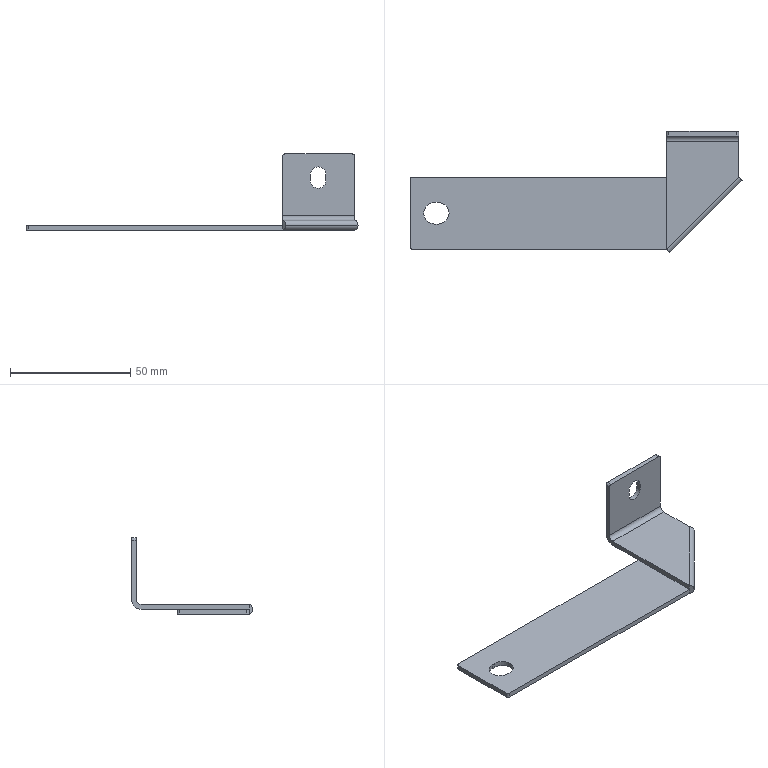Part | NX | features BREP 1 | 1 solid | 32 faces | box 138.159 x 50.414 x 31.629 mm | volume 10937 mm3 | plane 18 | cylinder 14 | commonest cylinder face diameters 2 x4 4 x3 6.5 x3 9 x3 8 x1
STEP:
#1=CARTESIAN_POINT('',(435.713,-98.404,2034.));
#2=VERTEX_POINT('',#1);
#3=CARTESIAN_POINT('',(437.128,-99.818,2036.));
#4=VERTEX_POINT('',#3);
#5=CARTESIAN_POINT('',(435.713,-98.404,2036.));
#6=DIRECTION('',(-0.7071,-0.7071,0.));
#7=DIRECTION('',(0.7071,-0.7071,0.));
#8=AXIS2_PLACEMENT_3D('',#5,#6,#7);
#9=CIRCLE('',#8,2.);
#10=EDGE_CURVE('',#2,#4,#9,.T.);
#11=ORIENTED_EDGE('',*,*,#10,.T.);
#12=CARTESIAN_POINT('',(407.128,-129.818,2036.));
#13=VERTEX_POINT('',#12);
#14=CARTESIAN_POINT('',(437.128,-99.818,2036.));
#15=DIRECTION('',(-0.7071,-0.7071,0.));
#16=VECTOR('',#15,1000.);
#17=LINE('',#14,#16);
#18=EDGE_CURVE('',#4,#13,#17,.T.);
#19=ORIENTED_EDGE('',*,*,#18,.T.);
#20=CARTESIAN_POINT('',(405.713,-128.404,2034.));
#21=VERTEX_POINT('',#20);
#22=CARTESIAN_POINT('',(405.713,-128.404,2036.));
#23=DIRECTION('',(0.7071,0.7071,0.));
#24=DIRECTION('',(0.7071,-0.7071,0.));
#25=AXIS2_PLACEMENT_3D('',#22,#23,#24);
#26=CIRCLE('',#25,2.);
#27=EDGE_CURVE('',#13,#21,#26,.T.);
#28=ORIENTED_EDGE('',*,*,#27,.T.);
#29=CARTESIAN_POINT('',(405.713,-128.404,2034.));
#30=DIRECTION('',(0.7071,0.7071,0.));
#31=VECTOR('',#30,1000.);
#32=LINE('',#29,#31);
#33=EDGE_CURVE('',#21,#2,#32,.T.);
#34=ORIENTED_EDGE('',*,*,#33,.T.);
#35=EDGE_LOOP('',(#11,#19,#28,#34));
#36=FACE_BOUND('',#35,.T.);
#37=CARTESIAN_POINT('',(435.713,-98.404,2036.));
#38=DIRECTION('',(-0.7071,-0.7071,0.));
#39=DIRECTION('',(-0.7071,0.7071,0.));
#40=AXIS2_PLACEMENT_3D('',#37,#38,#39);
#41=CYLINDRICAL_SURFACE('',#40,2.);
#42=ADVANCED_FACE('',(#36),#41,.T.);
#43=CARTESIAN_POINT('',(310.718,-108.904,2034.));
#44=VERTEX_POINT('',#43);
#45=CARTESIAN_POINT('',(315.218,-113.404,2034.));
#46=VERTEX_POINT('',#45);
#47=CARTESIAN_POINT('',(310.718,-113.404,2034.));
#48=DIRECTION('',(0.,0.,-1.));
#49=DIRECTION('',(1.,0.,0.));
#50=AXIS2_PLACEMENT_3D('',#47,#48,#49);
#51=CIRCLE('',#50,4.5);
#52=EDGE_CURVE('',#44,#46,#51,.T.);
#53=ORIENTED_EDGE('',*,*,#52,.T.);
#54=CARTESIAN_POINT('',(315.218,-113.404,2036.));
#55=VERTEX_POINT('',#54);
#56=CARTESIAN_POINT('',(315.218,-113.404,2016.46));
#57=DIRECTION('',(0.,0.,1.));
#58=VECTOR('',#57,1000.);
#59=LINE('',#56,#58);
#60=EDGE_CURVE('',#46,#55,#59,.T.);
#61=ORIENTED_EDGE('',*,*,#60,.T.);
#62=CARTESIAN_POINT('',(310.718,-108.904,2036.));
#63=VERTEX_POINT('',#62);
#64=CARTESIAN_POINT('',(310.718,-113.404,2036.));
#65=DIRECTION('',(0.,0.,-1.));
#66=DIRECTION('',(1.,0.,0.));
#67=AXIS2_PLACEMENT_3D('',#64,#65,#66);
#68=CIRCLE('',#67,4.5);
#69=EDGE_CURVE('',#63,#55,#68,.T.);
#70=ORIENTED_EDGE('',*,*,#69,.F.);
#71=CARTESIAN_POINT('',(310.718,-108.904,2016.46));
#72=DIRECTION('',(0.,0.,1.));
#73=VECTOR('',#72,1000.);
#74=LINE('',#71,#73);
#75=EDGE_CURVE('',#44,#63,#74,.T.);
#76=ORIENTED_EDGE('',*,*,#75,.F.);
#77=EDGE_LOOP('',(#53,#61,#70,#76));
#78=FACE_BOUND('',#77,.T.);
#79=CARTESIAN_POINT('',(310.718,-113.404,2016.46));
#80=DIRECTION('',(0.,0.,1.));
#81=DIRECTION('',(-1.,0.,0.));
#82=AXIS2_PLACEMENT_3D('',#79,#80,#81);
#83=CYLINDRICAL_SURFACE('',#82,4.5);
#84=ADVANCED_FACE('',(#78),#83,.F.);
#85=CARTESIAN_POINT('',(423.779,-81.404,2057.042));
#86=VERTEX_POINT('',#85);
#87=CARTESIAN_POINT('',(420.529,-81.404,2060.292));
#88=VERTEX_POINT('',#87);
#89=CARTESIAN_POINT('',(420.529,-81.404,2057.042));
#90=DIRECTION('',(0.,-1.,0.));
#91=DIRECTION('',(0.,0.,1.));
#92=AXIS2_PLACEMENT_3D('',#89,#90,#91);
#93=CIRCLE('',#92,3.25);
#94=EDGE_CURVE('',#86,#88,#93,.T.);
#95=ORIENTED_EDGE('',*,*,#94,.T.);
#96=CARTESIAN_POINT('',(420.529,-79.404,2060.292));
#97=VERTEX_POINT('',#96);
#98=CARTESIAN_POINT('',(420.529,-80.404,2060.292));
#99=DIRECTION('',(0.,1.,0.));
#100=VECTOR('',#99,1000.);
#101=LINE('',#98,#100);
#102=EDGE_CURVE('',#88,#97,#101,.T.);
#103=ORIENTED_EDGE('',*,*,#102,.T.);
#104=CARTESIAN_POINT('',(423.779,-79.404,2057.042));
#105=VERTEX_POINT('',#104);
#106=CARTESIAN_POINT('',(420.529,-79.404,2057.042));
#107=DIRECTION('',(0.,-1.,0.));
#108=DIRECTION('',(0.,0.,1.));
#109=AXIS2_PLACEMENT_3D('',#106,#107,#108);
#110=CIRCLE('',#109,3.25);
#111=EDGE_CURVE('',#105,#97,#110,.T.);
#112=ORIENTED_EDGE('',*,*,#111,.F.);
#113=CARTESIAN_POINT('',(423.779,-80.404,2057.042));
#114=DIRECTION('',(0.,1.,0.));
#115=VECTOR('',#114,1000.);
#116=LINE('',#113,#115);
#117=EDGE_CURVE('',#86,#105,#116,.T.);
#118=ORIENTED_EDGE('',*,*,#117,.F.);
#119=EDGE_LOOP('',(#95,#103,#112,#118));
#120=FACE_BOUND('',#119,.T.);
#121=CARTESIAN_POINT('',(420.529,-80.404,2057.042));
#122=DIRECTION('',(0.,1.,0.));
#123=DIRECTION('',(0.,0.,-1.));
#124=AXIS2_PLACEMENT_3D('',#121,#122,#123);
#125=CYLINDRICAL_SURFACE('',#124,3.25);
#126=ADVANCED_FACE('',(#120),#125,.F.);
#127=CARTESIAN_POINT('',(298.968,-99.404,2034.));
#128=VERTEX_POINT('',#127);
#129=CARTESIAN_POINT('',(298.968,-127.404,2034.));
#130=VERTEX_POINT('',#129);
#131=CARTESIAN_POINT('',(298.968,-6.11,2034.));
#132=DIRECTION('',(0.,-1.,0.));
#133=VECTOR('',#132,1000.);
#134=LINE('',#131,#133);
#135=EDGE_CURVE('',#128,#130,#134,.T.);
#136=ORIENTED_EDGE('',*,*,#135,.F.);
#137=CARTESIAN_POINT('',(299.968,-98.404,2034.));
#138=VERTEX_POINT('',#137);
#139=CARTESIAN_POINT('',(299.968,-99.404,2034.));
#140=DIRECTION('',(0.,0.,1.));
#141=DIRECTION('',(1.,0.,0.));
#142=AXIS2_PLACEMENT_3D('',#139,#140,#141);
#143=CIRCLE('',#142,1.);
#144=EDGE_CURVE('',#138,#128,#143,.T.);
#145=ORIENTED_EDGE('',*,*,#144,.F.);
#146=CARTESIAN_POINT('',(-23.45,-98.404,2034.));
#147=DIRECTION('',(-1.,0.,0.));
#148=VECTOR('',#147,1000.);
#149=LINE('',#146,#148);
#150=EDGE_CURVE('',#2,#138,#149,.T.);
#151=ORIENTED_EDGE('',*,*,#150,.F.);
#152=ORIENTED_EDGE('',*,*,#33,.F.);
#153=CARTESIAN_POINT('',(299.968,-128.404,2034.));
#154=VERTEX_POINT('',#153);
#155=CARTESIAN_POINT('',(-23.45,-128.404,2034.));
#156=DIRECTION('',(1.,0.,0.));
#157=VECTOR('',#156,1000.);
#158=LINE('',#155,#157);
#159=EDGE_CURVE('',#154,#21,#158,.T.);
#160=ORIENTED_EDGE('',*,*,#159,.F.);
#161=CARTESIAN_POINT('',(299.968,-127.404,2034.));
#162=DIRECTION('',(0.,0.,1.));
#163=DIRECTION('',(1.,0.,0.));
#164=AXIS2_PLACEMENT_3D('',#161,#162,#163);
#165=CIRCLE('',#164,1.);
#166=EDGE_CURVE('',#130,#154,#165,.T.);
#167=ORIENTED_EDGE('',*,*,#166,.F.);
#168=EDGE_LOOP('',(#136,#145,#151,#152,#160,#167));
#169=FACE_BOUND('',#168,.T.);
#170=CARTESIAN_POINT('',(309.218,-117.904,2034.));
#171=VERTEX_POINT('',#170);
#172=CARTESIAN_POINT('',(310.718,-117.904,2034.));
#173=VERTEX_POINT('',#172);
#174=CARTESIAN_POINT('',(309.218,-117.904,2034.));
#175=DIRECTION('',(1.,0.,0.));
#176=VECTOR('',#175,1000.);
#177=LINE('',#174,#176);
#178=EDGE_CURVE('',#171,#173,#177,.T.);
#179=ORIENTED_EDGE('',*,*,#178,.T.);
#180=CARTESIAN_POINT('',(310.718,-113.404,2034.));
#181=DIRECTION('',(0.,0.,-1.));
#182=DIRECTION('',(1.,0.,0.));
#183=AXIS2_PLACEMENT_3D('',#180,#181,#182);
#184=CIRCLE('',#183,4.5);
#185=EDGE_CURVE('',#46,#173,#184,.T.);
#186=ORIENTED_EDGE('',*,*,#185,.F.);
#187=ORIENTED_EDGE('',*,*,#52,.F.);
#188=CARTESIAN_POINT('',(309.218,-108.904,2034.));
#189=VERTEX_POINT('',#188);
#190=CARTESIAN_POINT('',(310.718,-108.904,2034.));
#191=DIRECTION('',(-1.,0.,0.));
#192=VECTOR('',#191,1000.);
#193=LINE('',#190,#192);
#194=EDGE_CURVE('',#44,#189,#193,.T.);
#195=ORIENTED_EDGE('',*,*,#194,.T.);
#196=CARTESIAN_POINT('',(309.218,-113.404,2034.));
#197=DIRECTION('',(0.,0.,-1.));
#198=DIRECTION('',(1.,0.,0.));
#199=AXIS2_PLACEMENT_3D('',#196,#197,#198);
#200=CIRCLE('',#199,4.5);
#201=EDGE_CURVE('',#171,#189,#200,.T.);
#202=ORIENTED_EDGE('',*,*,#201,.F.);
#203=EDGE_LOOP('',(#179,#186,#187,#195,#202));
#204=FACE_BOUND('',#203,.T.);
#205=CARTESIAN_POINT('',(-23.45,-6.11,2034.));
#206=DIRECTION('',(0.,0.,1.));
#207=DIRECTION('',(-1.,0.,0.));
#208=AXIS2_PLACEMENT_3D('',#205,#206,#207);
#209=PLANE('',#208);
#210=ADVANCED_FACE('',(#169,#204),#209,.F.);
#211=ORIENTED_EDGE('',*,*,#135,.T.);
#212=CARTESIAN_POINT('',(298.968,-127.404,2036.));
#213=VERTEX_POINT('',#212);
#214=CARTESIAN_POINT('',(298.968,-127.404,2035.));
#215=DIRECTION('',(0.,0.,1.));
#216=VECTOR('',#215,1000.);
#217=LINE('',#214,#216);
#218=EDGE_CURVE('',#130,#213,#217,.T.);
#219=ORIENTED_EDGE('',*,*,#218,.T.);
#220=CARTESIAN_POINT('',(298.968,-99.404,2036.));
#221=VERTEX_POINT('',#220);
#222=CARTESIAN_POINT('',(298.968,-113.404,2036.));
#223=DIRECTION('',(0.,1.,0.));
#224=VECTOR('',#223,1000.);
#225=LINE('',#222,#224);
#226=EDGE_CURVE('',#213,#221,#225,.T.);
#227=ORIENTED_EDGE('',*,*,#226,.T.);
#228=CARTESIAN_POINT('',(298.968,-99.404,2035.));
#229=DIRECTION('',(0.,0.,-1.));
#230=VECTOR('',#229,1000.);
#231=LINE('',#228,#230);
#232=EDGE_CURVE('',#221,#128,#231,.T.);
#233=ORIENTED_EDGE('',*,*,#232,.T.);
#234=EDGE_LOOP('',(#211,#219,#227,#233));
#235=FACE_BOUND('',#234,.T.);
#236=CARTESIAN_POINT('',(298.968,-113.404,2035.));
#237=DIRECTION('',(-1.,0.,0.));
#238=DIRECTION('',(0.,0.,-1.));
#239=AXIS2_PLACEMENT_3D('',#236,#237,#238);
#240=PLANE('',#239);
#241=ADVANCED_FACE('',(#235),#240,.T.);
#242=CARTESIAN_POINT('',(405.713,-98.404,2036.));
#243=VERTEX_POINT('',#242);
#244=CARTESIAN_POINT('',(435.713,-98.404,2036.));
#245=VERTEX_POINT('',#244);
#246=CARTESIAN_POINT('',(339.341,-98.404,2036.));
#247=DIRECTION('',(1.,0.,0.));
#248=VECTOR('',#247,1000.);
#249=LINE('',#246,#248);
#250=EDGE_CURVE('',#243,#245,#249,.T.);
#251=ORIENTED_EDGE('',*,*,#250,.T.);
#252=CARTESIAN_POINT('',(435.713,-98.404,2035.));
#253=DIRECTION('',(0.,0.,-1.));
#254=VECTOR('',#253,1000.);
#255=LINE('',#252,#254);
#256=EDGE_CURVE('',#245,#2,#255,.T.);
#257=ORIENTED_EDGE('',*,*,#256,.T.);
#258=ORIENTED_EDGE('',*,*,#150,.T.);
#259=CARTESIAN_POINT('',(299.968,-98.404,2036.));
#260=VERTEX_POINT('',#259);
#261=CARTESIAN_POINT('',(299.968,-98.404,2035.));
#262=DIRECTION('',(0.,0.,1.));
#263=VECTOR('',#262,1000.);
#264=LINE('',#261,#263);
#265=EDGE_CURVE('',#138,#260,#264,.T.);
#266=ORIENTED_EDGE('',*,*,#265,.T.);
#267=CARTESIAN_POINT('',(339.341,-98.404,2036.));
#268=DIRECTION('',(1.,0.,0.));
#269=VECTOR('',#268,1000.);
#270=LINE('',#267,#269);
#271=EDGE_CURVE('',#260,#243,#270,.T.);
#272=ORIENTED_EDGE('',*,*,#271,.T.);
#273=EDGE_LOOP('',(#251,#257,#258,#266,#272));
#274=FACE_BOUND('',#273,.T.);
#275=CARTESIAN_POINT('',(339.341,-98.404,2035.));
#276=DIRECTION('',(0.,1.,0.));
#277=DIRECTION('',(0.,0.,-1.));
#278=AXIS2_PLACEMENT_3D('',#275,#276,#277);
#279=PLANE('',#278);
#280=ADVANCED_FACE('',(#274),#279,.T.);
#281=ORIENTED_EDGE('',*,*,#18,.F.);
#282=CARTESIAN_POINT('',(435.713,-98.404,2038.));
#283=VERTEX_POINT('',#282);
#284=CARTESIAN_POINT('',(435.713,-98.404,2036.));
#285=DIRECTION('',(-0.7071,-0.7071,0.));
#286=DIRECTION('',(0.7071,-0.7071,0.));
#287=AXIS2_PLACEMENT_3D('',#284,#285,#286);
#288=CIRCLE('',#287,2.);
#289=EDGE_CURVE('',#4,#283,#288,.T.);
#290=ORIENTED_EDGE('',*,*,#289,.T.);
#291=CARTESIAN_POINT('',(405.713,-128.404,2038.));
#292=VERTEX_POINT('',#291);
#293=CARTESIAN_POINT('',(435.713,-98.404,2038.));
#294=DIRECTION('',(-0.7071,-0.7071,0.));
#295=VECTOR('',#294,1000.);
#296=LINE('',#293,#295);
#297=EDGE_CURVE('',#283,#292,#296,.T.);
#298=ORIENTED_EDGE('',*,*,#297,.T.);
#299=CARTESIAN_POINT('',(405.713,-128.404,2036.));
#300=DIRECTION('',(0.7071,0.7071,0.));
#301=DIRECTION('',(0.7071,-0.7071,0.));
#302=AXIS2_PLACEMENT_3D('',#299,#300,#301);
#303=CIRCLE('',#302,2.);
#304=EDGE_CURVE('',#292,#13,#303,.T.);
#305=ORIENTED_EDGE('',*,*,#304,.T.);
#306=EDGE_LOOP('',(#281,#290,#298,#305));
#307=FACE_BOUND('',#306,.T.);
#308=CARTESIAN_POINT('',(435.713,-98.404,2036.));
#309=DIRECTION('',(-0.7071,-0.7071,0.));
#310=DIRECTION('',(-0.7071,0.7071,0.));
#311=AXIS2_PLACEMENT_3D('',#308,#309,#310);
#312=CYLINDRICAL_SURFACE('',#311,2.);
#313=ADVANCED_FACE('',(#307),#312,.T.);
#314=ORIENTED_EDGE('',*,*,#159,.T.);
#315=CARTESIAN_POINT('',(405.713,-128.404,2036.));
#316=VERTEX_POINT('',#315);
#317=CARTESIAN_POINT('',(405.713,-128.404,2035.));
#318=DIRECTION('',(0.,0.,1.));
#319=VECTOR('',#318,1000.);
#320=LINE('',#317,#319);
#321=EDGE_CURVE('',#21,#316,#320,.T.);
#322=ORIENTED_EDGE('',*,*,#321,.T.);
#323=CARTESIAN_POINT('',(299.968,-128.404,2036.));
#324=VERTEX_POINT('',#323);
#325=CARTESIAN_POINT('',(339.341,-128.404,2036.));
#326=DIRECTION('',(-1.,0.,0.));
#327=VECTOR('',#326,1000.);
#328=LINE('',#325,#327);
#329=EDGE_CURVE('',#316,#324,#328,.T.);
#330=ORIENTED_EDGE('',*,*,#329,.T.);
#331=CARTESIAN_POINT('',(299.968,-128.404,2035.));
#332=DIRECTION('',(0.,0.,-1.));
#333=VECTOR('',#332,1000.);
#334=LINE('',#331,#333);
#335=EDGE_CURVE('',#324,#154,#334,.T.);
#336=ORIENTED_EDGE('',*,*,#335,.T.);
#337=EDGE_LOOP('',(#314,#322,#330,#336));
#338=FACE_BOUND('',#337,.T.);
#339=CARTESIAN_POINT('',(339.341,-128.404,2035.));
#340=DIRECTION('',(0.,-1.,0.));
#341=DIRECTION('',(0.,0.,1.));
#342=AXIS2_PLACEMENT_3D('',#339,#340,#341);
#343=PLANE('',#342);
#344=ADVANCED_FACE('',(#338),#343,.T.);
#345=ORIENTED_EDGE('',*,*,#60,.F.);
#346=ORIENTED_EDGE('',*,*,#185,.T.);
#347=CARTESIAN_POINT('',(310.718,-117.904,2036.));
#348=VERTEX_POINT('',#347);
#349=CARTESIAN_POINT('',(310.718,-117.904,2016.46));
#350=DIRECTION('',(0.,0.,-1.));
#351=VECTOR('',#350,1000.);
#352=LINE('',#349,#351);
#353=EDGE_CURVE('',#348,#173,#352,.T.);
#354=ORIENTED_EDGE('',*,*,#353,.F.);
#355=CARTESIAN_POINT('',(310.718,-113.404,2036.));
#356=DIRECTION('',(0.,0.,-1.));
#357=DIRECTION('',(1.,0.,0.));
#358=AXIS2_PLACEMENT_3D('',#355,#356,#357);
#359=CIRCLE('',#358,4.5);
#360=EDGE_CURVE('',#55,#348,#359,.T.);
#361=ORIENTED_EDGE('',*,*,#360,.F.);
#362=EDGE_LOOP('',(#345,#346,#354,#361));
#363=FACE_BOUND('',#362,.T.);
#364=CARTESIAN_POINT('',(310.718,-113.404,2016.46));
#365=DIRECTION('',(0.,0.,1.));
#366=DIRECTION('',(-1.,0.,0.));
#367=AXIS2_PLACEMENT_3D('',#364,#365,#366);
#368=CYLINDRICAL_SURFACE('',#367,4.5);
#369=ADVANCED_FACE('',(#363),#368,.F.);
#370=ORIENTED_EDGE('',*,*,#201,.T.);
#371=CARTESIAN_POINT('',(309.218,-108.904,2036.));
#372=VERTEX_POINT('',#371);
#373=CARTESIAN_POINT('',(309.218,-108.904,2016.46));
#374=DIRECTION('',(0.,0.,-1.));
#375=VECTOR('',#374,1000.);
#376=LINE('',#373,#375);
#377=EDGE_CURVE('',#372,#189,#376,.T.);
#378=ORIENTED_EDGE('',*,*,#377,.F.);
#379=CARTESIAN_POINT('',(309.218,-117.904,2036.));
#380=VERTEX_POINT('',#379);
#381=CARTESIAN_POINT('',(309.218,-113.404,2036.));
#382=DIRECTION('',(0.,0.,-1.));
#383=DIRECTION('',(1.,0.,0.));
#384=AXIS2_PLACEMENT_3D('',#381,#382,#383);
#385=CIRCLE('',#384,4.5);
#386=EDGE_CURVE('',#380,#372,#385,.T.);
#387=ORIENTED_EDGE('',*,*,#386,.F.);
#388=CARTESIAN_POINT('',(309.218,-117.904,2016.46));
#389=DIRECTION('',(0.,0.,1.));
#390=VECTOR('',#389,1000.);
#391=LINE('',#388,#390);
#392=EDGE_CURVE('',#171,#380,#391,.T.);
#393=ORIENTED_EDGE('',*,*,#392,.F.);
#394=EDGE_LOOP('',(#370,#378,#387,#393));
#395=FACE_BOUND('',#394,.T.);
#396=CARTESIAN_POINT('',(309.218,-113.404,2016.46));
#397=DIRECTION('',(0.,0.,1.));
#398=DIRECTION('',(-1.,0.,0.));
#399=AXIS2_PLACEMENT_3D('',#396,#397,#398);
#400=CYLINDRICAL_SURFACE('',#399,4.5);
#401=ADVANCED_FACE('',(#395),#400,.F.);
#402=ORIENTED_EDGE('',*,*,#218,.F.);
#403=ORIENTED_EDGE('',*,*,#166,.T.);
#404=ORIENTED_EDGE('',*,*,#335,.F.);
#405=CARTESIAN_POINT('',(299.968,-127.404,2036.));
#406=DIRECTION('',(0.,0.,-1.));
#407=DIRECTION('',(1.,0.,0.));
#408=AXIS2_PLACEMENT_3D('',#405,#406,#407);
#409=CIRCLE('',#408,1.);
#410=EDGE_CURVE('',#324,#213,#409,.T.);
#411=ORIENTED_EDGE('',*,*,#410,.T.);
#412=EDGE_LOOP('',(#402,#403,#404,#411));
#413=FACE_BOUND('',#412,.T.);
#414=CARTESIAN_POINT('',(299.968,-127.404,1963.606));
#415=DIRECTION('',(0.,0.,1.));
#416=DIRECTION('',(-1.,0.,0.));
#417=AXIS2_PLACEMENT_3D('',#414,#415,#416);
#418=CYLINDRICAL_SURFACE('',#417,1.);
#419=ADVANCED_FACE('',(#413),#418,.T.);
#420=ORIENTED_EDGE('',*,*,#265,.F.);
#421=ORIENTED_EDGE('',*,*,#144,.T.);
#422=ORIENTED_EDGE('',*,*,#232,.F.);
#423=CARTESIAN_POINT('',(299.968,-99.404,2036.));
#424=DIRECTION('',(0.,0.,-1.));
#425=DIRECTION('',(1.,0.,0.));
#426=AXIS2_PLACEMENT_3D('',#423,#424,#425);
#427=CIRCLE('',#426,1.);
#428=EDGE_CURVE('',#221,#260,#427,.T.);
#429=ORIENTED_EDGE('',*,*,#428,.T.);
#430=EDGE_LOOP('',(#420,#421,#422,#429));
#431=FACE_BOUND('',#430,.T.);
#432=CARTESIAN_POINT('',(299.968,-99.404,1963.606));
#433=DIRECTION('',(0.,0.,1.));
#434=DIRECTION('',(-1.,0.,0.));
#435=AXIS2_PLACEMENT_3D('',#432,#433,#434);
#436=CYLINDRICAL_SURFACE('',#435,1.);
#437=ADVANCED_FACE('',(#431),#436,.T.);
#438=ORIENTED_EDGE('',*,*,#271,.F.);
#439=ORIENTED_EDGE('',*,*,#428,.F.);
#440=ORIENTED_EDGE('',*,*,#226,.F.);
#441=ORIENTED_EDGE('',*,*,#410,.F.);
#442=ORIENTED_EDGE('',*,*,#329,.F.);
#443=CARTESIAN_POINT('',(405.713,-6.11,2036.));
#444=DIRECTION('',(0.,1.,0.));
#445=VECTOR('',#444,1000.);
#446=LINE('',#443,#445);
#447=EDGE_CURVE('',#316,#243,#446,.T.);
#448=ORIENTED_EDGE('',*,*,#447,.T.);
#449=EDGE_LOOP('',(#438,#439,#440,#441,#442,#448));
#450=FACE_BOUND('',#449,.T.);
#451=CARTESIAN_POINT('',(7.55,-117.904,2036.));
#452=DIRECTION('',(-1.,0.,0.));
#453=VECTOR('',#452,1000.);
#454=LINE('',#451,#453);
#455=EDGE_CURVE('',#348,#380,#454,.T.);
#456=ORIENTED_EDGE('',*,*,#455,.T.);
#457=ORIENTED_EDGE('',*,*,#386,.T.);
#458=CARTESIAN_POINT('',(7.55,-108.904,2036.));
#459=DIRECTION('',(1.,0.,0.));
#460=VECTOR('',#459,1000.);
#461=LINE('',#458,#460);
#462=EDGE_CURVE('',#372,#63,#461,.T.);
#463=ORIENTED_EDGE('',*,*,#462,.T.);
#464=ORIENTED_EDGE('',*,*,#69,.T.);
#465=ORIENTED_EDGE('',*,*,#360,.T.);
#466=EDGE_LOOP('',(#456,#457,#463,#464,#465));
#467=FACE_BOUND('',#466,.T.);
#468=CARTESIAN_POINT('',(7.55,-6.11,2036.));
#469=DIRECTION('',(0.,0.,1.));
#470=DIRECTION('',(-1.,0.,0.));
#471=AXIS2_PLACEMENT_3D('',#468,#469,#470);
#472=PLANE('',#471);
#473=ADVANCED_FACE('',(#450,#467),#472,.T.);
#474=CARTESIAN_POINT('',(435.713,-98.404,2036.));
#475=DIRECTION('',(0.,0.,1.));
#476=VECTOR('',#475,1000.);
#477=LINE('',#474,#476);
#478=EDGE_CURVE('',#245,#283,#477,.T.);
#479=ORIENTED_EDGE('',*,*,#478,.T.);
#480=ORIENTED_EDGE('',*,*,#289,.F.);
#481=ORIENTED_EDGE('',*,*,#10,.F.);
#482=ORIENTED_EDGE('',*,*,#256,.F.);
#483=EDGE_LOOP('',(#479,#480,#481,#482));
#484=FACE_BOUND('',#483,.T.);
#485=CARTESIAN_POINT('',(436.42,-99.111,2036.));
#486=DIRECTION('',(0.7071,0.7071,0.));
#487=DIRECTION('',(0.7071,-0.7071,0.));
#488=AXIS2_PLACEMENT_3D('',#485,#486,#487);
#489=PLANE('',#488);
#490=ADVANCED_FACE('',(#484),#489,.T.);
#491=CARTESIAN_POINT('',(435.713,-83.404,2036.));
#492=VERTEX_POINT('',#491);
#493=CARTESIAN_POINT('',(435.713,-6.11,2036.));
#494=DIRECTION('',(0.,1.,0.));
#495=VECTOR('',#494,1000.);
#496=LINE('',#493,#495);
#497=EDGE_CURVE('',#245,#492,#496,.T.);
#498=ORIENTED_EDGE('',*,*,#497,.F.);
#499=ORIENTED_EDGE('',*,*,#250,.F.);
#500=CARTESIAN_POINT('',(405.713,-83.404,2036.));
#501=VERTEX_POINT('',#500);
#502=CARTESIAN_POINT('',(405.713,-6.11,2036.));
#503=DIRECTION('',(0.,-1.,0.));
#504=VECTOR('',#503,1000.);
#505=LINE('',#502,#504);
#506=EDGE_CURVE('',#501,#243,#505,.T.);
#507=ORIENTED_EDGE('',*,*,#506,.F.);
#508=CARTESIAN_POINT('',(7.55,-83.404,2036.));
#509=DIRECTION('',(-1.,0.,0.));
#510=VECTOR('',#509,1000.);
#511=LINE('',#508,#510);
#512=EDGE_CURVE('',#492,#501,#511,.T.);
#513=ORIENTED_EDGE('',*,*,#512,.F.);
#514=EDGE_LOOP('',(#498,#499,#507,#513));
#515=FACE_BOUND('',#514,.T.);
#516=CARTESIAN_POINT('',(7.55,-6.11,2036.));
#517=DIRECTION('',(0.,0.,1.));
#518=DIRECTION('',(-1.,0.,0.));
#519=AXIS2_PLACEMENT_3D('',#516,#517,#518);
#520=PLANE('',#519);
#521=ADVANCED_FACE('',(#515),#520,.F.);
#522=ORIENTED_EDGE('',*,*,#304,.F.);
#523=CARTESIAN_POINT('',(405.713,-128.404,2036.));
#524=DIRECTION('',(0.,0.,-1.));
#525=VECTOR('',#524,1000.);
#526=LINE('',#523,#525);
#527=EDGE_CURVE('',#292,#316,#526,.T.);
#528=ORIENTED_EDGE('',*,*,#527,.T.);
#529=ORIENTED_EDGE('',*,*,#321,.F.);
#530=ORIENTED_EDGE('',*,*,#27,.F.);
#531=EDGE_LOOP('',(#522,#528,#529,#530));
#532=FACE_BOUND('',#531,.T.);
#533=CARTESIAN_POINT('',(406.42,-129.111,2036.));
#534=DIRECTION('',(-0.7071,-0.7071,0.));
#535=DIRECTION('',(-0.7071,0.7071,0.));
#536=AXIS2_PLACEMENT_3D('',#533,#534,#535);
#537=PLANE('',#536);
#538=ADVANCED_FACE('',(#532),#537,.T.);
#539=ORIENTED_EDGE('',*,*,#353,.T.);
#540=ORIENTED_EDGE('',*,*,#178,.F.);
#541=ORIENTED_EDGE('',*,*,#392,.T.);
#542=ORIENTED_EDGE('',*,*,#455,.F.);
#543=EDGE_LOOP('',(#539,#540,#541,#542));
#544=FACE_BOUND('',#543,.T.);
#545=CARTESIAN_POINT('',(309.218,-117.904,2016.46));
#546=DIRECTION('',(0.,-1.,0.));
#547=DIRECTION('',(0.,0.,1.));
#548=AXIS2_PLACEMENT_3D('',#545,#546,#547);
#549=PLANE('',#548);
#550=ADVANCED_FACE('',(#544),#549,.F.);
#551=ORIENTED_EDGE('',*,*,#377,.T.);
#552=ORIENTED_EDGE('',*,*,#194,.F.);
#553=ORIENTED_EDGE('',*,*,#75,.T.);
#554=ORIENTED_EDGE('',*,*,#462,.F.);
#555=EDGE_LOOP('',(#551,#552,#553,#554));
#556=FACE_BOUND('',#555,.T.);
#557=CARTESIAN_POINT('',(310.718,-108.904,2016.46));
#558=DIRECTION('',(0.,1.,0.));
#559=DIRECTION('',(0.,0.,-1.));
#560=AXIS2_PLACEMENT_3D('',#557,#558,#559);
#561=PLANE('',#560);
#562=ADVANCED_FACE('',(#556),#561,.F.);
#563=CARTESIAN_POINT('',(405.713,-83.404,2038.));
#564=VERTEX_POINT('',#563);
#565=CARTESIAN_POINT('',(405.713,-103.904,2038.));
#566=DIRECTION('',(0.,1.,0.));
#567=VECTOR('',#566,1000.);
#568=LINE('',#565,#567);
#569=EDGE_CURVE('',#292,#564,#568,.T.);
#570=ORIENTED_EDGE('',*,*,#569,.T.);
#571=CARTESIAN_POINT('',(405.713,-81.404,2040.));
#572=VERTEX_POINT('',#571);
#573=CARTESIAN_POINT('',(405.713,-83.404,2040.));
#574=DIRECTION('',(1.,0.,0.));
#575=DIRECTION('',(0.,0.,1.));
#576=AXIS2_PLACEMENT_3D('',#573,#574,#575);
#577=CIRCLE('',#576,2.);
#578=EDGE_CURVE('',#564,#572,#577,.T.);
#579=ORIENTED_EDGE('',*,*,#578,.T.);
#580=CARTESIAN_POINT('',(405.713,-81.404,2064.629));
#581=VERTEX_POINT('',#580);
#582=CARTESIAN_POINT('',(405.713,-81.404,2034.5));
#583=DIRECTION('',(0.,0.,1.));
#584=VECTOR('',#583,1000.);
#585=LINE('',#582,#584);
#586=EDGE_CURVE('',#572,#581,#585,.T.);
#587=ORIENTED_EDGE('',*,*,#586,.T.);
#588=CARTESIAN_POINT('',(405.713,-79.404,2064.629));
#589=VERTEX_POINT('',#588);
#590=CARTESIAN_POINT('',(405.713,-103.904,2064.629));
#591=DIRECTION('',(0.,1.,0.));
#592=VECTOR('',#591,1000.);
#593=LINE('',#590,#592);
#594=EDGE_CURVE('',#581,#589,#593,.T.);
#595=ORIENTED_EDGE('',*,*,#594,.T.);
#596=CARTESIAN_POINT('',(405.713,-79.404,2040.));
#597=VERTEX_POINT('',#596);
#598=CARTESIAN_POINT('',(405.713,-79.404,2034.5));
#599=DIRECTION('',(0.,0.,-1.));
#600=VECTOR('',#599,1000.);
#601=LINE('',#598,#600);
#602=EDGE_CURVE('',#589,#597,#601,.T.);
#603=ORIENTED_EDGE('',*,*,#602,.T.);
#604=CARTESIAN_POINT('',(405.713,-83.404,2040.));
#605=DIRECTION('',(-1.,0.,0.));
#606=DIRECTION('',(0.,0.,1.));
#607=AXIS2_PLACEMENT_3D('',#604,#605,#606);
#608=CIRCLE('',#607,4.);
#609=EDGE_CURVE('',#597,#501,#608,.T.);
#610=ORIENTED_EDGE('',*,*,#609,.T.);
#611=ORIENTED_EDGE('',*,*,#506,.T.);
#612=ORIENTED_EDGE('',*,*,#447,.F.);
#613=ORIENTED_EDGE('',*,*,#527,.F.);
#614=EDGE_LOOP('',(#570,#579,#587,#595,#603,#610,#611,#612,#613));
#615=FACE_BOUND('',#614,.T.);
#616=CARTESIAN_POINT('',(405.713,-103.904,2034.5));
#617=DIRECTION('',(-1.,0.,0.));
#618=DIRECTION('',(0.,0.,-1.));
#619=AXIS2_PLACEMENT_3D('',#616,#617,#618);
#620=PLANE('',#619);
#621=ADVANCED_FACE('',(#615),#620,.T.);
#622=CARTESIAN_POINT('',(435.713,-83.404,2038.));
#623=VERTEX_POINT('',#622);
#624=CARTESIAN_POINT('',(435.713,-88.904,2038.));
#625=DIRECTION('',(0.,-1.,0.));
#626=VECTOR('',#625,1000.);
#627=LINE('',#624,#626);
#628=EDGE_CURVE('',#623,#283,#627,.T.);
#629=ORIENTED_EDGE('',*,*,#628,.T.);
#630=ORIENTED_EDGE('',*,*,#478,.F.);
#631=ORIENTED_EDGE('',*,*,#497,.T.);
#632=CARTESIAN_POINT('',(435.713,-79.404,2040.));
#633=VERTEX_POINT('',#632);
#634=CARTESIAN_POINT('',(435.713,-83.404,2040.));
#635=DIRECTION('',(1.,0.,0.));
#636=DIRECTION('',(0.,0.,1.));
#637=AXIS2_PLACEMENT_3D('',#634,#635,#636);
#638=CIRCLE('',#637,4.);
#639=EDGE_CURVE('',#492,#633,#638,.T.);
#640=ORIENTED_EDGE('',*,*,#639,.T.);
#641=CARTESIAN_POINT('',(435.713,-79.404,2064.629));
#642=VERTEX_POINT('',#641);
#643=CARTESIAN_POINT('',(435.713,-79.404,2034.5));
#644=DIRECTION('',(0.,0.,1.));
#645=VECTOR('',#644,1000.);
#646=LINE('',#643,#645);
#647=EDGE_CURVE('',#633,#642,#646,.T.);
#648=ORIENTED_EDGE('',*,*,#647,.T.);
#649=CARTESIAN_POINT('',(435.713,-81.404,2064.629));
#650=VERTEX_POINT('',#649);
#651=CARTESIAN_POINT('',(435.713,-88.904,2064.629));
#652=DIRECTION('',(0.,-1.,0.));
#653=VECTOR('',#652,1000.);
#654=LINE('',#651,#653);
#655=EDGE_CURVE('',#642,#650,#654,.T.);
#656=ORIENTED_EDGE('',*,*,#655,.T.);
#657=CARTESIAN_POINT('',(435.713,-81.404,2040.));
#658=VERTEX_POINT('',#657);
#659=CARTESIAN_POINT('',(435.713,-81.404,2034.5));
#660=DIRECTION('',(0.,0.,-1.));
#661=VECTOR('',#660,1000.);
#662=LINE('',#659,#661);
#663=EDGE_CURVE('',#650,#658,#662,.T.);
#664=ORIENTED_EDGE('',*,*,#663,.T.);
#665=CARTESIAN_POINT('',(435.713,-83.404,2040.));
#666=DIRECTION('',(-1.,0.,0.));
#667=DIRECTION('',(0.,0.,1.));
#668=AXIS2_PLACEMENT_3D('',#665,#666,#667);
#669=CIRCLE('',#668,2.);
#670=EDGE_CURVE('',#658,#623,#669,.T.);
#671=ORIENTED_EDGE('',*,*,#670,.T.);
#672=EDGE_LOOP('',(#629,#630,#631,#640,#648,#656,#664,#671));
#673=FACE_BOUND('',#672,.T.);
#674=CARTESIAN_POINT('',(435.713,-88.904,2034.5));
#675=DIRECTION('',(1.,0.,0.));
#676=DIRECTION('',(0.,0.,1.));
#677=AXIS2_PLACEMENT_3D('',#674,#675,#676);
#678=PLANE('',#677);
#679=ADVANCED_FACE('',(#673),#678,.T.);
#680=ORIENTED_EDGE('',*,*,#512,.T.);
#681=ORIENTED_EDGE('',*,*,#609,.F.);
#682=CARTESIAN_POINT('',(435.713,-79.404,2040.));
#683=DIRECTION('',(1.,0.,0.));
#684=VECTOR('',#683,1000.);
#685=LINE('',#682,#684);
#686=EDGE_CURVE('',#597,#633,#685,.T.);
#687=ORIENTED_EDGE('',*,*,#686,.T.);
#688=ORIENTED_EDGE('',*,*,#639,.F.);
#689=EDGE_LOOP('',(#680,#681,#687,#688));
#690=FACE_BOUND('',#689,.T.);
#691=CARTESIAN_POINT('',(435.713,-83.404,2040.));
#692=DIRECTION('',(-1.,0.,0.));
#693=DIRECTION('',(0.,0.,-1.));
#694=AXIS2_PLACEMENT_3D('',#691,#692,#693);
#695=CYLINDRICAL_SURFACE('',#694,4.);
#696=ADVANCED_FACE('',(#690),#695,.T.);
#697=ORIENTED_EDGE('',*,*,#297,.F.);
#698=ORIENTED_EDGE('',*,*,#628,.F.);
#699=CARTESIAN_POINT('',(412.841,-83.404,2038.));
#700=DIRECTION('',(1.,0.,0.));
#701=VECTOR('',#700,1000.);
#702=LINE('',#699,#701);
#703=EDGE_CURVE('',#564,#623,#702,.T.);
#704=ORIENTED_EDGE('',*,*,#703,.F.);
#705=ORIENTED_EDGE('',*,*,#569,.F.);
#706=EDGE_LOOP('',(#697,#698,#704,#705));
#707=FACE_BOUND('',#706,.T.);
#708=CARTESIAN_POINT('',(412.841,-121.276,2038.));
#709=DIRECTION('',(0.,0.,-1.));
#710=DIRECTION('',(1.,0.,0.));
#711=AXIS2_PLACEMENT_3D('',#708,#709,#710);
#712=PLANE('',#711);
#713=ADVANCED_FACE('',(#707),#712,.F.);
#714=ORIENTED_EDGE('',*,*,#578,.F.);
#715=ORIENTED_EDGE('',*,*,#703,.T.);
#716=ORIENTED_EDGE('',*,*,#670,.F.);
#717=CARTESIAN_POINT('',(435.713,-81.404,2040.));
#718=DIRECTION('',(1.,0.,0.));
#719=VECTOR('',#718,1000.);
#720=LINE('',#717,#719);
#721=EDGE_CURVE('',#572,#658,#720,.T.);
#722=ORIENTED_EDGE('',*,*,#721,.F.);
#723=EDGE_LOOP('',(#714,#715,#716,#722));
#724=FACE_BOUND('',#723,.T.);
#725=CARTESIAN_POINT('',(435.713,-83.404,2040.));
#726=DIRECTION('',(-1.,0.,0.));
#727=DIRECTION('',(0.,0.,-1.));
#728=AXIS2_PLACEMENT_3D('',#725,#726,#727);
#729=CYLINDRICAL_SURFACE('',#728,2.);
#730=ADVANCED_FACE('',(#724),#729,.F.);
#731=ORIENTED_EDGE('',*,*,#602,.F.);
#732=CARTESIAN_POINT('',(406.713,-79.404,2065.629));
#733=VERTEX_POINT('',#732);
#734=CARTESIAN_POINT('',(406.713,-79.404,2064.629));
#735=DIRECTION('',(0.,1.,0.));
#736=DIRECTION('',(0.,0.,-1.));
#737=AXIS2_PLACEMENT_3D('',#734,#735,#736);
#738=CIRCLE('',#737,1.);
#739=EDGE_CURVE('',#589,#733,#738,.T.);
#740=ORIENTED_EDGE('',*,*,#739,.T.);
#741=CARTESIAN_POINT('',(434.713,-79.404,2065.629));
#742=VERTEX_POINT('',#741);
#743=CARTESIAN_POINT('',(405.713,-79.404,2065.629));
#744=DIRECTION('',(1.,0.,0.));
#745=VECTOR('',#744,1000.);
#746=LINE('',#743,#745);
#747=EDGE_CURVE('',#733,#742,#746,.T.);
#748=ORIENTED_EDGE('',*,*,#747,.T.);
#749=CARTESIAN_POINT('',(434.713,-79.404,2064.629));
#750=DIRECTION('',(0.,1.,0.));
#751=DIRECTION('',(0.,0.,1.));
#752=AXIS2_PLACEMENT_3D('',#749,#750,#751);
#753=CIRCLE('',#752,1.);
#754=EDGE_CURVE('',#742,#642,#753,.T.);
#755=ORIENTED_EDGE('',*,*,#754,.T.);
#756=ORIENTED_EDGE('',*,*,#647,.F.);
#757=ORIENTED_EDGE('',*,*,#686,.F.);
#758=EDGE_LOOP('',(#731,#740,#748,#755,#756,#757));
#759=FACE_BOUND('',#758,.T.);
#760=CARTESIAN_POINT('',(417.279,-79.404,2057.042));
#761=VERTEX_POINT('',#760);
#762=CARTESIAN_POINT('',(417.279,-79.404,2054.542));
#763=VERTEX_POINT('',#762);
#764=CARTESIAN_POINT('',(417.279,-79.404,2033.5));
#765=DIRECTION('',(0.,0.,-1.));
#766=VECTOR('',#765,1000.);
#767=LINE('',#764,#766);
#768=EDGE_CURVE('',#761,#763,#767,.T.);
#769=ORIENTED_EDGE('',*,*,#768,.T.);
#770=CARTESIAN_POINT('',(423.779,-79.404,2054.542));
#771=VERTEX_POINT('',#770);
#772=CARTESIAN_POINT('',(420.529,-79.404,2054.542));
#773=DIRECTION('',(0.,-1.,0.));
#774=DIRECTION('',(0.,0.,1.));
#775=AXIS2_PLACEMENT_3D('',#772,#773,#774);
#776=CIRCLE('',#775,3.25);
#777=EDGE_CURVE('',#763,#771,#776,.T.);
#778=ORIENTED_EDGE('',*,*,#777,.T.);
#779=CARTESIAN_POINT('',(423.779,-79.404,2033.5));
#780=DIRECTION('',(0.,0.,1.));
#781=VECTOR('',#780,1000.);
#782=LINE('',#779,#781);
#783=EDGE_CURVE('',#771,#105,#782,.T.);
#784=ORIENTED_EDGE('',*,*,#783,.T.);
#785=ORIENTED_EDGE('',*,*,#111,.T.);
#786=CARTESIAN_POINT('',(420.529,-79.404,2057.042));
#787=DIRECTION('',(0.,-1.,0.));
#788=DIRECTION('',(0.,0.,1.));
#789=AXIS2_PLACEMENT_3D('',#786,#787,#788);
#790=CIRCLE('',#789,3.25);
#791=EDGE_CURVE('',#97,#761,#790,.T.);
#792=ORIENTED_EDGE('',*,*,#791,.T.);
#793=EDGE_LOOP('',(#769,#778,#784,#785,#792));
#794=FACE_BOUND('',#793,.T.);
#795=CARTESIAN_POINT('',(405.713,-79.404,2033.5));
#796=DIRECTION('',(0.,1.,0.));
#797=DIRECTION('',(0.,0.,-1.));
#798=AXIS2_PLACEMENT_3D('',#795,#796,#797);
#799=PLANE('',#798);
#800=ADVANCED_FACE('',(#759,#794),#799,.T.);
#801=CARTESIAN_POINT('',(406.713,-81.404,2065.629));
#802=VERTEX_POINT('',#801);
#803=CARTESIAN_POINT('',(406.713,-81.404,2064.629));
#804=DIRECTION('',(0.,1.,0.));
#805=DIRECTION('',(0.,0.,-1.));
#806=AXIS2_PLACEMENT_3D('',#803,#804,#805);
#807=CIRCLE('',#806,1.);
#808=EDGE_CURVE('',#581,#802,#807,.T.);
#809=ORIENTED_EDGE('',*,*,#808,.T.);
#810=CARTESIAN_POINT('',(406.713,-103.904,2065.629));
#811=DIRECTION('',(0.,1.,0.));
#812=VECTOR('',#811,1000.);
#813=LINE('',#810,#812);
#814=EDGE_CURVE('',#802,#733,#813,.T.);
#815=ORIENTED_EDGE('',*,*,#814,.T.);
#816=ORIENTED_EDGE('',*,*,#739,.F.);
#817=ORIENTED_EDGE('',*,*,#594,.F.);
#818=EDGE_LOOP('',(#809,#815,#816,#817));
#819=FACE_BOUND('',#818,.T.);
#820=CARTESIAN_POINT('',(406.713,-103.904,2064.629));
#821=DIRECTION('',(0.,-1.,0.));
#822=DIRECTION('',(0.,0.,1.));
#823=AXIS2_PLACEMENT_3D('',#820,#821,#822);
#824=CYLINDRICAL_SURFACE('',#823,1.);
#825=ADVANCED_FACE('',(#819),#824,.T.);
#826=ORIENTED_EDGE('',*,*,#808,.F.);
#827=ORIENTED_EDGE('',*,*,#586,.F.);
#828=ORIENTED_EDGE('',*,*,#721,.T.);
#829=ORIENTED_EDGE('',*,*,#663,.F.);
#830=CARTESIAN_POINT('',(434.713,-81.404,2065.629));
#831=VERTEX_POINT('',#830);
#832=CARTESIAN_POINT('',(434.713,-81.404,2064.629));
#833=DIRECTION('',(0.,1.,0.));
#834=DIRECTION('',(0.,0.,1.));
#835=AXIS2_PLACEMENT_3D('',#832,#833,#834);
#836=CIRCLE('',#835,1.);
#837=EDGE_CURVE('',#831,#650,#836,.T.);
#838=ORIENTED_EDGE('',*,*,#837,.F.);
#839=CARTESIAN_POINT('',(405.713,-81.404,2065.629));
#840=DIRECTION('',(1.,0.,0.));
#841=VECTOR('',#840,1000.);
#842=LINE('',#839,#841);
#843=EDGE_CURVE('',#802,#831,#842,.T.);
#844=ORIENTED_EDGE('',*,*,#843,.F.);
#845=EDGE_LOOP('',(#826,#827,#828,#829,#838,#844));
#846=FACE_BOUND('',#845,.T.);
#847=CARTESIAN_POINT('',(417.279,-81.404,2057.042));
#848=VERTEX_POINT('',#847);
#849=CARTESIAN_POINT('',(417.279,-81.404,2054.542));
#850=VERTEX_POINT('',#849);
#851=CARTESIAN_POINT('',(417.279,-81.404,2033.5));
#852=DIRECTION('',(0.,0.,-1.));
#853=VECTOR('',#852,1000.);
#854=LINE('',#851,#853);
#855=EDGE_CURVE('',#848,#850,#854,.T.);
#856=ORIENTED_EDGE('',*,*,#855,.F.);
#857=CARTESIAN_POINT('',(420.529,-81.404,2057.042));
#858=DIRECTION('',(0.,-1.,0.));
#859=DIRECTION('',(0.,0.,1.));
#860=AXIS2_PLACEMENT_3D('',#857,#858,#859);
#861=CIRCLE('',#860,3.25);
#862=EDGE_CURVE('',#88,#848,#861,.T.);
#863=ORIENTED_EDGE('',*,*,#862,.F.);
#864=ORIENTED_EDGE('',*,*,#94,.F.);
#865=CARTESIAN_POINT('',(423.779,-81.404,2054.542));
#866=VERTEX_POINT('',#865);
#867=CARTESIAN_POINT('',(423.779,-81.404,2033.5));
#868=DIRECTION('',(0.,0.,1.));
#869=VECTOR('',#868,1000.);
#870=LINE('',#867,#869);
#871=EDGE_CURVE('',#866,#86,#870,.T.);
#872=ORIENTED_EDGE('',*,*,#871,.F.);
#873=CARTESIAN_POINT('',(420.529,-81.404,2054.542));
#874=DIRECTION('',(0.,-1.,0.));
#875=DIRECTION('',(0.,0.,1.));
#876=AXIS2_PLACEMENT_3D('',#873,#874,#875);
#877=CIRCLE('',#876,3.25);
#878=EDGE_CURVE('',#850,#866,#877,.T.);
#879=ORIENTED_EDGE('',*,*,#878,.F.);
#880=EDGE_LOOP('',(#856,#863,#864,#872,#879));
#881=FACE_BOUND('',#880,.T.);
#882=CARTESIAN_POINT('',(405.713,-81.404,2033.5));
#883=DIRECTION('',(0.,1.,0.));
#884=DIRECTION('',(0.,0.,-1.));
#885=AXIS2_PLACEMENT_3D('',#882,#883,#884);
#886=PLANE('',#885);
#887=ADVANCED_FACE('',(#846,#881),#886,.F.);
#888=ORIENTED_EDGE('',*,*,#754,.F.);
#889=CARTESIAN_POINT('',(434.713,-80.404,2065.629));
#890=DIRECTION('',(0.,-1.,0.));
#891=VECTOR('',#890,1000.);
#892=LINE('',#889,#891);
#893=EDGE_CURVE('',#742,#831,#892,.T.);
#894=ORIENTED_EDGE('',*,*,#893,.T.);
#895=ORIENTED_EDGE('',*,*,#837,.T.);
#896=ORIENTED_EDGE('',*,*,#655,.F.);
#897=EDGE_LOOP('',(#888,#894,#895,#896));
#898=FACE_BOUND('',#897,.T.);
#899=CARTESIAN_POINT('',(434.713,-80.404,2064.629));
#900=DIRECTION('',(0.,1.,0.));
#901=DIRECTION('',(0.,0.,-1.));
#902=AXIS2_PLACEMENT_3D('',#899,#900,#901);
#903=CYLINDRICAL_SURFACE('',#902,1.);
#904=ADVANCED_FACE('',(#898),#903,.T.);
#905=ORIENTED_EDGE('',*,*,#747,.F.);
#906=ORIENTED_EDGE('',*,*,#814,.F.);
#907=ORIENTED_EDGE('',*,*,#843,.T.);
#908=ORIENTED_EDGE('',*,*,#893,.F.);
#909=EDGE_LOOP('',(#905,#906,#907,#908));
#910=FACE_BOUND('',#909,.T.);
#911=CARTESIAN_POINT('',(420.713,-80.404,2065.629));
#912=DIRECTION('',(0.,0.,1.));
#913=DIRECTION('',(-1.,0.,0.));
#914=AXIS2_PLACEMENT_3D('',#911,#912,#913);
#915=PLANE('',#914);
#916=ADVANCED_FACE('',(#910),#915,.T.);
#917=CARTESIAN_POINT('',(417.279,-80.404,2054.542));
#918=DIRECTION('',(0.,1.,0.));
#919=VECTOR('',#918,1000.);
#920=LINE('',#917,#919);
#921=EDGE_CURVE('',#850,#763,#920,.T.);
#922=ORIENTED_EDGE('',*,*,#921,.F.);
#923=ORIENTED_EDGE('',*,*,#878,.T.);
#924=CARTESIAN_POINT('',(423.779,-80.404,2054.542));
#925=DIRECTION('',(0.,-1.,0.));
#926=VECTOR('',#925,1000.);
#927=LINE('',#924,#926);
#928=EDGE_CURVE('',#771,#866,#927,.T.);
#929=ORIENTED_EDGE('',*,*,#928,.F.);
#930=ORIENTED_EDGE('',*,*,#777,.F.);
#931=EDGE_LOOP('',(#922,#923,#929,#930));
#932=FACE_BOUND('',#931,.T.);
#933=CARTESIAN_POINT('',(420.529,-80.404,2054.542));
#934=DIRECTION('',(0.,1.,0.));
#935=DIRECTION('',(0.,0.,-1.));
#936=AXIS2_PLACEMENT_3D('',#933,#934,#935);
#937=CYLINDRICAL_SURFACE('',#936,3.25);
#938=ADVANCED_FACE('',(#932),#937,.F.);
#939=ORIENTED_EDGE('',*,*,#768,.F.);
#940=CARTESIAN_POINT('',(417.279,-81.404,2057.042));
#941=DIRECTION('',(0.,-1.,0.));
#942=VECTOR('',#941,1000.);
#943=LINE('',#940,#942);
#944=EDGE_CURVE('',#761,#848,#943,.T.);
#945=ORIENTED_EDGE('',*,*,#944,.T.);
#946=ORIENTED_EDGE('',*,*,#855,.T.);
#947=ORIENTED_EDGE('',*,*,#921,.T.);
#948=EDGE_LOOP('',(#939,#945,#946,#947));
#949=FACE_BOUND('',#948,.T.);
#950=CARTESIAN_POINT('',(417.279,-81.404,2060.292));
#951=DIRECTION('',(1.,0.,0.));
#952=DIRECTION('',(0.,0.,1.));
#953=AXIS2_PLACEMENT_3D('',#950,#951,#952);
#954=PLANE('',#953);
#955=ADVANCED_FACE('',(#949),#954,.T.);
#956=ORIENTED_EDGE('',*,*,#102,.F.);
#957=ORIENTED_EDGE('',*,*,#862,.T.);
#958=ORIENTED_EDGE('',*,*,#944,.F.);
#959=ORIENTED_EDGE('',*,*,#791,.F.);
#960=EDGE_LOOP('',(#956,#957,#958,#959));
#961=FACE_BOUND('',#960,.T.);
#962=CARTESIAN_POINT('',(420.529,-80.404,2057.042));
#963=DIRECTION('',(0.,1.,0.));
#964=DIRECTION('',(0.,0.,-1.));
#965=AXIS2_PLACEMENT_3D('',#962,#963,#964);
#966=CYLINDRICAL_SURFACE('',#965,3.25);
#967=ADVANCED_FACE('',(#961),#966,.F.);
#968=ORIENTED_EDGE('',*,*,#871,.T.);
#969=ORIENTED_EDGE('',*,*,#117,.T.);
#970=ORIENTED_EDGE('',*,*,#783,.F.);
#971=ORIENTED_EDGE('',*,*,#928,.T.);
#972=EDGE_LOOP('',(#968,#969,#970,#971));
#973=FACE_BOUND('',#972,.T.);
#974=CARTESIAN_POINT('',(423.779,-81.404,2051.292));
#975=DIRECTION('',(-1.,0.,0.));
#976=DIRECTION('',(0.,0.,-1.));
#977=AXIS2_PLACEMENT_3D('',#974,#975,#976);
#978=PLANE('',#977);
#979=ADVANCED_FACE('',(#973),#978,.T.);
#980=CLOSED_SHELL('',(#42,#84,#126,#210,#241,#280,#313,#344,#369,#401,#419,#437,#473,#490,#521,#538,#550,#562,#621,#679,#696,#713,#730,#800,#825,#887,#904,#916,#938,#955,#967,#979));
#981=MANIFOLD_SOLID_BREP('',#980);
#982=(LENGTH_UNIT()NAMED_UNIT(*)SI_UNIT(.MILLI.,.METRE.));
#983=UNCERTAINTY_MEASURE_WITH_UNIT(LENGTH_MEASURE(0.00001),#982,'','');
#984=(NAMED_UNIT(*)PLANE_ANGLE_UNIT()SI_UNIT($,.RADIAN.));
#985=(NAMED_UNIT(*)SI_UNIT($,.STERADIAN.)SOLID_ANGLE_UNIT());
#986=(GEOMETRIC_REPRESENTATION_CONTEXT(3)GLOBAL_UNCERTAINTY_ASSIGNED_CONTEXT((#983))GLOBAL_UNIT_ASSIGNED_CONTEXT((#982,#984,#985))REPRESENTATION_CONTEXT('',''));
#987=ADVANCED_BREP_SHAPE_REPRESENTATION('',(#981),#986);